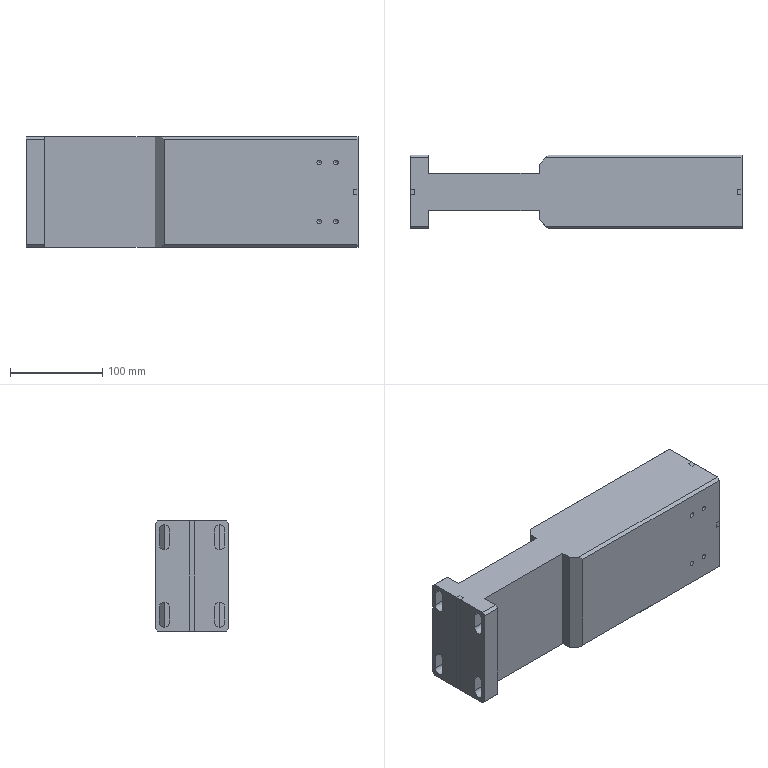Part | 2 solids | 156 faces | box 360 x 80 x 120 mm | volume 5662131 mm3 | plane 80 | cylinder 46 | cone 30 | commonest cylinder face diameters 5 x16 11 x16 6.8 x8 3.3 x6